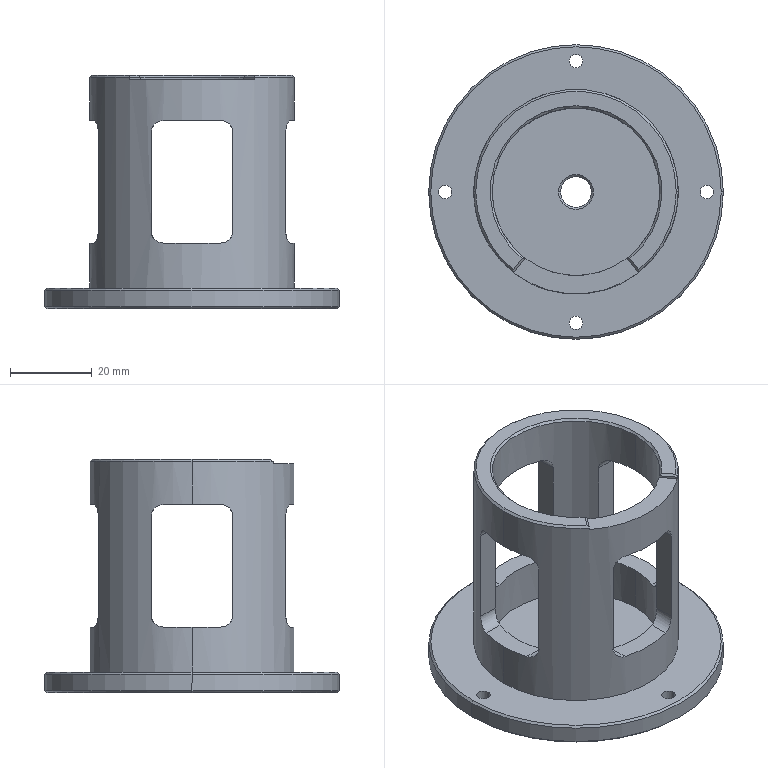Part | STEP file | Outer collar ring | 1 solid | 69 faces | box 72 x 72 x 57 mm | volume 42154 mm3 | cylinder 32 | plane 25 | cone 12 | commonest cylinder face diameters 6 x16 3.3 x8 7.5 x2 41 x2 50 x2 72 x2